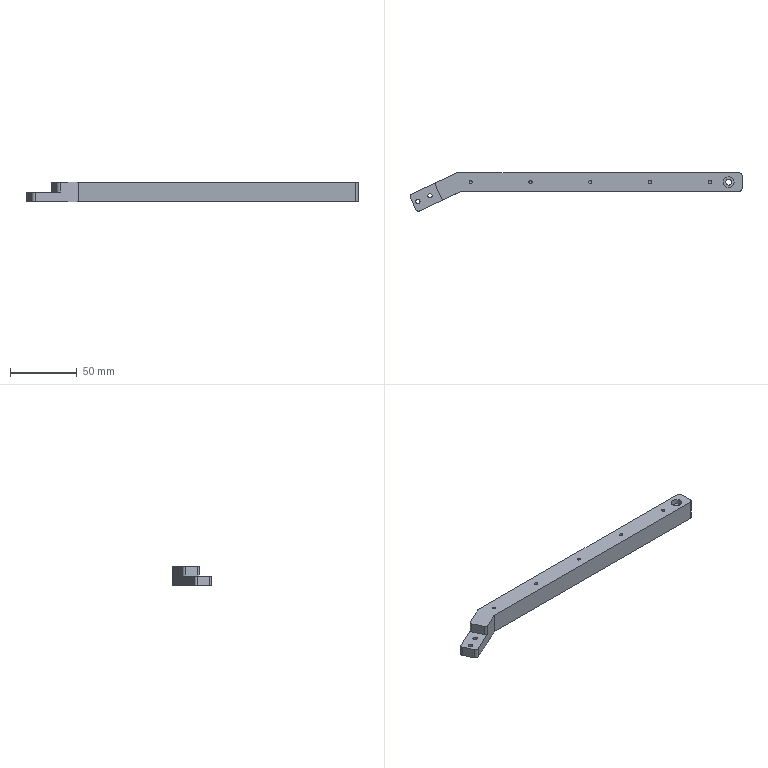Part | NX | 1 solid | 33 faces | box 249.594 x 28.935 x 15 mm | volume 49736 mm3 | cylinder 17 | plane 11 | cone 5 | commonest cylinder face diameters 4 x8 2.459 x5 3.242 x2 4.5 x1 8 x1
STEP:
#1=CARTESIAN_POINT('',(-120.493,-7.091,-15.));
#2=VERTEX_POINT('',#1);
#3=CARTESIAN_POINT('',(-118.872,-7.091,-15.));
#4=DIRECTION('',(0.,0.,1.));
#5=DIRECTION('',(-1.,0.,0.));
#6=AXIS2_PLACEMENT_3D('',#3,#4,#5);
#7=CIRCLE('',#6,1.621);
#8=EDGE_CURVE('',#2,#2,#7,.T.);
#9=ORIENTED_EDGE('',*,*,#8,.F.);
#10=EDGE_LOOP('',(#9));
#11=FACE_BOUND('',#10,.T.);
#12=CARTESIAN_POINT('',(-120.493,-7.091,-7.5));
#13=VERTEX_POINT('',#12);
#14=CARTESIAN_POINT('',(-118.872,-7.091,-7.5));
#15=DIRECTION('',(0.,0.,1.));
#16=DIRECTION('',(-1.,0.,0.));
#17=AXIS2_PLACEMENT_3D('',#14,#15,#16);
#18=CIRCLE('',#17,1.621);
#19=EDGE_CURVE('',#13,#13,#18,.T.);
#20=ORIENTED_EDGE('',*,*,#19,.T.);
#21=EDGE_LOOP('',(#20));
#22=FACE_BOUND('',#21,.T.);
#23=CARTESIAN_POINT('',(-118.872,-7.091,-7.5));
#24=DIRECTION('',(0.,0.,-1.));
#25=DIRECTION('',(0.,-1.,0.));
#26=AXIS2_PLACEMENT_3D('',#23,#24,#25);
#27=CYLINDRICAL_SURFACE('',#26,1.621);
#28=ADVANCED_FACE('',(#11,#22),#27,.F.);
#29=CARTESIAN_POINT('',(117.047,7.468,-15.));
#30=VERTEX_POINT('',#29);
#31=CARTESIAN_POINT('',(114.797,7.468,-15.));
#32=DIRECTION('',(0.,0.,-1.));
#33=DIRECTION('',(1.,0.,0.));
#34=AXIS2_PLACEMENT_3D('',#31,#32,#33);
#35=CIRCLE('',#34,2.25);
#36=EDGE_CURVE('',#30,#30,#35,.T.);
#37=ORIENTED_EDGE('',*,*,#36,.F.);
#38=EDGE_LOOP('',(#37));
#39=FACE_BOUND('',#38,.T.);
#40=CARTESIAN_POINT('',(-108.187,-2.865,-15.));
#41=VERTEX_POINT('',#40);
#42=CARTESIAN_POINT('',(-109.808,-2.865,-15.));
#43=DIRECTION('',(0.,0.,-1.));
#44=DIRECTION('',(1.,0.,0.));
#45=AXIS2_PLACEMENT_3D('',#42,#43,#44);
#46=CIRCLE('',#45,1.621);
#47=EDGE_CURVE('',#41,#41,#46,.T.);
#48=ORIENTED_EDGE('',*,*,#47,.F.);
#49=EDGE_LOOP('',(#48));
#50=FACE_BOUND('',#49,.T.);
#51=ORIENTED_EDGE('',*,*,#8,.T.);
#52=EDGE_LOOP('',(#51));
#53=FACE_BOUND('',#52,.T.);
#54=CARTESIAN_POINT('',(-86.501,0.2802,-15.));
#55=VERTEX_POINT('',#54);
#56=CARTESIAN_POINT('',(-117.726,-14.28,-15.));
#57=VERTEX_POINT('',#56);
#58=CARTESIAN_POINT('',(-102.113,-7.,-15.));
#59=DIRECTION('',(-0.9063,-0.4226,0.));
#60=VECTOR('',#59,1000.);
#61=LINE('',#58,#60);
#62=EDGE_CURVE('',#55,#57,#61,.T.);
#63=ORIENTED_EDGE('',*,*,#62,.T.);
#64=CARTESIAN_POINT('',(-120.384,-13.313,-15.));
#65=VERTEX_POINT('',#64);
#66=CARTESIAN_POINT('',(-118.571,-12.468,-15.));
#67=DIRECTION('',(0.,0.,-1.));
#68=DIRECTION('',(1.,0.,0.));
#69=AXIS2_PLACEMENT_3D('',#66,#67,#68);
#70=CIRCLE('',#69,2.);
#71=EDGE_CURVE('',#57,#65,#70,.T.);
#72=ORIENTED_EDGE('',*,*,#71,.T.);
#73=CARTESIAN_POINT('',(-124.61,-4.25,-15.));
#74=VERTEX_POINT('',#73);
#75=CARTESIAN_POINT('',(-122.497,-8.781,-15.));
#76=DIRECTION('',(0.4226,-0.9063,0.));
#77=VECTOR('',#76,1000.);
#78=LINE('',#75,#77);
#79=EDGE_CURVE('',#74,#65,#78,.T.);
#80=ORIENTED_EDGE('',*,*,#79,.F.);
#81=CARTESIAN_POINT('',(-123.642,-1.592,-15.));
#82=VERTEX_POINT('',#81);
#83=CARTESIAN_POINT('',(-122.797,-3.405,-15.));
#84=DIRECTION('',(0.,0.,-1.));
#85=DIRECTION('',(1.,0.,0.));
#86=AXIS2_PLACEMENT_3D('',#83,#84,#85);
#87=CIRCLE('',#86,2.);
#88=EDGE_CURVE('',#74,#82,#87,.T.);
#89=ORIENTED_EDGE('',*,*,#88,.T.);
#90=CARTESIAN_POINT('',(-89.605,14.28,-15.));
#91=VERTEX_POINT('',#90);
#92=CARTESIAN_POINT('',(-106.624,6.344,-15.));
#93=DIRECTION('',(0.9063,0.4226,0.));
#94=VECTOR('',#93,1000.);
#95=LINE('',#92,#94);
#96=EDGE_CURVE('',#82,#91,#95,.T.);
#97=ORIENTED_EDGE('',*,*,#96,.T.);
#98=CARTESIAN_POINT('',(-88.759,14.468,-15.));
#99=VERTEX_POINT('',#98);
#100=CARTESIAN_POINT('',(-88.759,12.468,-15.));
#101=DIRECTION('',(0.,0.,1.));
#102=DIRECTION('',(-1.,0.,0.));
#103=AXIS2_PLACEMENT_3D('',#100,#101,#102);
#104=CIRCLE('',#103,2.);
#105=EDGE_CURVE('',#99,#91,#104,.T.);
#106=ORIENTED_EDGE('',*,*,#105,.F.);
#107=CARTESIAN_POINT('',(122.797,14.468,-15.));
#108=VERTEX_POINT('',#107);
#109=CARTESIAN_POINT('',(17.019,14.468,-15.));
#110=DIRECTION('',(-1.,0.,0.));
#111=VECTOR('',#110,1000.);
#112=LINE('',#109,#111);
#113=EDGE_CURVE('',#108,#99,#112,.T.);
#114=ORIENTED_EDGE('',*,*,#113,.F.);
#115=CARTESIAN_POINT('',(124.797,12.468,-15.));
#116=VERTEX_POINT('',#115);
#117=CARTESIAN_POINT('',(122.797,12.468,-15.));
#118=DIRECTION('',(0.,0.,1.));
#119=DIRECTION('',(-1.,0.,0.));
#120=AXIS2_PLACEMENT_3D('',#117,#118,#119);
#121=CIRCLE('',#120,2.);
#122=EDGE_CURVE('',#116,#108,#121,.T.);
#123=ORIENTED_EDGE('',*,*,#122,.F.);
#124=CARTESIAN_POINT('',(124.797,2.468,-15.));
#125=VERTEX_POINT('',#124);
#126=CARTESIAN_POINT('',(124.797,7.468,-15.));
#127=DIRECTION('',(0.,1.,0.));
#128=VECTOR('',#127,1000.);
#129=LINE('',#126,#128);
#130=EDGE_CURVE('',#125,#116,#129,.T.);
#131=ORIENTED_EDGE('',*,*,#130,.F.);
#132=CARTESIAN_POINT('',(122.797,0.4676,-15.));
#133=VERTEX_POINT('',#132);
#134=CARTESIAN_POINT('',(122.797,2.468,-15.));
#135=DIRECTION('',(0.,0.,1.));
#136=DIRECTION('',(-1.,0.,0.));
#137=AXIS2_PLACEMENT_3D('',#134,#135,#136);
#138=CIRCLE('',#137,2.);
#139=EDGE_CURVE('',#133,#125,#138,.T.);
#140=ORIENTED_EDGE('',*,*,#139,.F.);
#141=CARTESIAN_POINT('',(-85.656,0.4676,-15.));
#142=VERTEX_POINT('',#141);
#143=CARTESIAN_POINT('',(18.571,0.4676,-15.));
#144=DIRECTION('',(1.,0.,0.));
#145=VECTOR('',#144,1000.);
#146=LINE('',#143,#145);
#147=EDGE_CURVE('',#142,#133,#146,.T.);
#148=ORIENTED_EDGE('',*,*,#147,.F.);
#149=CARTESIAN_POINT('',(-85.656,-1.532,-15.));
#150=DIRECTION('',(0.,0.,-1.));
#151=DIRECTION('',(1.,0.,0.));
#152=AXIS2_PLACEMENT_3D('',#149,#150,#151);
#153=CIRCLE('',#152,2.);
#154=EDGE_CURVE('',#55,#142,#153,.T.);
#155=ORIENTED_EDGE('',*,*,#154,.F.);
#156=EDGE_LOOP('',(#63,#72,#80,#89,#97,#106,#114,#123,#131,#140,#148,#155));
#157=FACE_BOUND('',#156,.T.);
#158=CARTESIAN_POINT('',(-89.203,14.468,-15.));
#159=DIRECTION('',(0.,0.,1.));
#160=DIRECTION('',(0.,-1.,0.));
#161=AXIS2_PLACEMENT_3D('',#158,#159,#160);
#162=PLANE('',#161);
#163=ADVANCED_FACE('',(#39,#50,#53,#157),#162,.F.);
#164=ORIENTED_EDGE('',*,*,#147,.T.);
#165=CARTESIAN_POINT('',(122.797,0.4676,0.));
#166=VERTEX_POINT('',#165);
#167=CARTESIAN_POINT('',(122.797,0.4676,-7.5));
#168=DIRECTION('',(0.,0.,1.));
#169=VECTOR('',#168,1000.);
#170=LINE('',#167,#169);
#171=EDGE_CURVE('',#133,#166,#170,.T.);
#172=ORIENTED_EDGE('',*,*,#171,.T.);
#173=CARTESIAN_POINT('',(-85.656,0.4676,0.));
#174=VERTEX_POINT('',#173);
#175=CARTESIAN_POINT('',(18.571,0.4676,0.));
#176=DIRECTION('',(1.,0.,0.));
#177=VECTOR('',#176,1000.);
#178=LINE('',#175,#177);
#179=EDGE_CURVE('',#174,#166,#178,.T.);
#180=ORIENTED_EDGE('',*,*,#179,.F.);
#181=CARTESIAN_POINT('',(-85.656,0.4676,-7.5));
#182=DIRECTION('',(0.,0.,-1.));
#183=VECTOR('',#182,1000.);
#184=LINE('',#181,#183);
#185=EDGE_CURVE('',#174,#142,#184,.T.);
#186=ORIENTED_EDGE('',*,*,#185,.T.);
#187=EDGE_LOOP('',(#164,#172,#180,#186));
#188=FACE_BOUND('',#187,.T.);
#189=CARTESIAN_POINT('',(-89.203,0.4676,-15.));
#190=DIRECTION('',(0.,-1.,0.));
#191=DIRECTION('',(1.,0.,0.));
#192=AXIS2_PLACEMENT_3D('',#189,#190,#191);
#193=PLANE('',#192);
#194=ADVANCED_FACE('',(#188),#193,.T.);
#195=CARTESIAN_POINT('',(102.027,7.468,0.));
#196=VERTEX_POINT('',#195);
#197=CARTESIAN_POINT('',(100.797,7.468,0.));
#198=DIRECTION('',(0.,0.,-1.));
#199=DIRECTION('',(1.,0.,0.));
#200=AXIS2_PLACEMENT_3D('',#197,#198,#199);
#201=CIRCLE('',#200,1.23);
#202=EDGE_CURVE('',#196,#196,#201,.T.);
#203=ORIENTED_EDGE('',*,*,#202,.T.);
#204=EDGE_LOOP('',(#203));
#205=FACE_BOUND('',#204,.T.);
#206=CARTESIAN_POINT('',(57.027,7.468,0.));
#207=VERTEX_POINT('',#206);
#208=CARTESIAN_POINT('',(55.797,7.468,0.));
#209=DIRECTION('',(0.,0.,-1.));
#210=DIRECTION('',(1.,0.,0.));
#211=AXIS2_PLACEMENT_3D('',#208,#209,#210);
#212=CIRCLE('',#211,1.23);
#213=EDGE_CURVE('',#207,#207,#212,.T.);
#214=ORIENTED_EDGE('',*,*,#213,.T.);
#215=EDGE_LOOP('',(#214));
#216=FACE_BOUND('',#215,.T.);
#217=CARTESIAN_POINT('',(12.027,7.468,0.));
#218=VERTEX_POINT('',#217);
#219=CARTESIAN_POINT('',(10.797,7.468,0.));
#220=DIRECTION('',(0.,0.,-1.));
#221=DIRECTION('',(1.,0.,0.));
#222=AXIS2_PLACEMENT_3D('',#219,#220,#221);
#223=CIRCLE('',#222,1.23);
#224=EDGE_CURVE('',#218,#218,#223,.T.);
#225=ORIENTED_EDGE('',*,*,#224,.T.);
#226=EDGE_LOOP('',(#225));
#227=FACE_BOUND('',#226,.T.);
#228=CARTESIAN_POINT('',(-32.973,7.468,0.));
#229=VERTEX_POINT('',#228);
#230=CARTESIAN_POINT('',(-34.203,7.468,0.));
#231=DIRECTION('',(0.,0.,-1.));
#232=DIRECTION('',(1.,0.,0.));
#233=AXIS2_PLACEMENT_3D('',#230,#231,#232);
#234=CIRCLE('',#233,1.23);
#235=EDGE_CURVE('',#229,#229,#234,.T.);
#236=ORIENTED_EDGE('',*,*,#235,.T.);
#237=EDGE_LOOP('',(#236));
#238=FACE_BOUND('',#237,.T.);
#239=CARTESIAN_POINT('',(118.797,7.468,0.));
#240=VERTEX_POINT('',#239);
#241=CARTESIAN_POINT('',(114.797,7.468,0.));
#242=DIRECTION('',(0.,0.,-1.));
#243=DIRECTION('',(1.,0.,0.));
#244=AXIS2_PLACEMENT_3D('',#241,#242,#243);
#245=CIRCLE('',#244,4.);
#246=EDGE_CURVE('',#240,#240,#245,.T.);
#247=ORIENTED_EDGE('',*,*,#246,.T.);
#248=EDGE_LOOP('',(#247));
#249=FACE_BOUND('',#248,.T.);
#250=CARTESIAN_POINT('',(-77.973,7.468,0.));
#251=VERTEX_POINT('',#250);
#252=CARTESIAN_POINT('',(-79.203,7.468,0.));
#253=DIRECTION('',(0.,0.,-1.));
#254=DIRECTION('',(1.,0.,0.));
#255=AXIS2_PLACEMENT_3D('',#252,#253,#254);
#256=CIRCLE('',#255,1.23);
#257=EDGE_CURVE('',#251,#251,#256,.T.);
#258=ORIENTED_EDGE('',*,*,#257,.T.);
#259=EDGE_LOOP('',(#258));
#260=FACE_BOUND('',#259,.T.);
#261=CARTESIAN_POINT('',(-86.501,0.2802,0.));
#262=VERTEX_POINT('',#261);
#263=CARTESIAN_POINT('',(-85.656,-1.532,0.));
#264=DIRECTION('',(0.,0.,-1.));
#265=DIRECTION('',(1.,0.,0.));
#266=AXIS2_PLACEMENT_3D('',#263,#264,#265);
#267=CIRCLE('',#266,2.);
#268=EDGE_CURVE('',#262,#174,#267,.T.);
#269=ORIENTED_EDGE('',*,*,#268,.T.);
#270=ORIENTED_EDGE('',*,*,#179,.T.);
#271=CARTESIAN_POINT('',(124.797,2.468,0.));
#272=VERTEX_POINT('',#271);
#273=CARTESIAN_POINT('',(122.797,2.468,0.));
#274=DIRECTION('',(0.,0.,1.));
#275=DIRECTION('',(-1.,0.,0.));
#276=AXIS2_PLACEMENT_3D('',#273,#274,#275);
#277=CIRCLE('',#276,2.);
#278=EDGE_CURVE('',#166,#272,#277,.T.);
#279=ORIENTED_EDGE('',*,*,#278,.T.);
#280=CARTESIAN_POINT('',(124.797,12.468,0.));
#281=VERTEX_POINT('',#280);
#282=CARTESIAN_POINT('',(124.797,7.468,0.));
#283=DIRECTION('',(0.,1.,0.));
#284=VECTOR('',#283,1000.);
#285=LINE('',#282,#284);
#286=EDGE_CURVE('',#272,#281,#285,.T.);
#287=ORIENTED_EDGE('',*,*,#286,.T.);
#288=CARTESIAN_POINT('',(122.797,14.468,0.));
#289=VERTEX_POINT('',#288);
#290=CARTESIAN_POINT('',(122.797,12.468,0.));
#291=DIRECTION('',(0.,0.,1.));
#292=DIRECTION('',(-1.,0.,0.));
#293=AXIS2_PLACEMENT_3D('',#290,#291,#292);
#294=CIRCLE('',#293,2.);
#295=EDGE_CURVE('',#281,#289,#294,.T.);
#296=ORIENTED_EDGE('',*,*,#295,.T.);
#297=CARTESIAN_POINT('',(-88.759,14.468,0.));
#298=VERTEX_POINT('',#297);
#299=CARTESIAN_POINT('',(17.019,14.468,0.));
#300=DIRECTION('',(-1.,0.,0.));
#301=VECTOR('',#300,1000.);
#302=LINE('',#299,#301);
#303=EDGE_CURVE('',#289,#298,#302,.T.);
#304=ORIENTED_EDGE('',*,*,#303,.T.);
#305=CARTESIAN_POINT('',(-89.605,14.28,0.));
#306=VERTEX_POINT('',#305);
#307=CARTESIAN_POINT('',(-88.759,12.468,0.));
#308=DIRECTION('',(0.,0.,1.));
#309=DIRECTION('',(-1.,0.,0.));
#310=AXIS2_PLACEMENT_3D('',#307,#308,#309);
#311=CIRCLE('',#310,2.);
#312=EDGE_CURVE('',#298,#306,#311,.T.);
#313=ORIENTED_EDGE('',*,*,#312,.T.);
#314=CARTESIAN_POINT('',(-104.61,7.283,0.));
#315=VERTEX_POINT('',#314);
#316=CARTESIAN_POINT('',(-97.107,10.782,0.));
#317=DIRECTION('',(0.9063,0.4226,0.));
#318=VECTOR('',#317,1000.);
#319=LINE('',#316,#318);
#320=EDGE_CURVE('',#315,#306,#319,.T.);
#321=ORIENTED_EDGE('',*,*,#320,.F.);
#322=CARTESIAN_POINT('',(-105.577,4.625,0.));
#323=VERTEX_POINT('',#322);
#324=CARTESIAN_POINT('',(-103.765,5.47,0.));
#325=DIRECTION('',(0.,0.,-1.));
#326=DIRECTION('',(1.,0.,0.));
#327=AXIS2_PLACEMENT_3D('',#324,#325,#326);
#328=CIRCLE('',#327,2.);
#329=EDGE_CURVE('',#323,#315,#328,.T.);
#330=ORIENTED_EDGE('',*,*,#329,.F.);
#331=CARTESIAN_POINT('',(-101.351,-4.438,0.));
#332=VERTEX_POINT('',#331);
#333=CARTESIAN_POINT('',(-103.464,0.09369,0.));
#334=DIRECTION('',(0.4226,-0.9063,0.));
#335=VECTOR('',#334,1000.);
#336=LINE('',#333,#335);
#337=EDGE_CURVE('',#323,#332,#336,.T.);
#338=ORIENTED_EDGE('',*,*,#337,.T.);
#339=CARTESIAN_POINT('',(-98.693,-5.405,0.));
#340=VERTEX_POINT('',#339);
#341=CARTESIAN_POINT('',(-99.539,-3.593,0.));
#342=DIRECTION('',(0.,0.,-1.));
#343=DIRECTION('',(1.,0.,0.));
#344=AXIS2_PLACEMENT_3D('',#341,#342,#343);
#345=CIRCLE('',#344,2.);
#346=EDGE_CURVE('',#340,#332,#345,.T.);
#347=ORIENTED_EDGE('',*,*,#346,.F.);
#348=CARTESIAN_POINT('',(-92.597,-2.563,0.));
#349=DIRECTION('',(-0.9063,-0.4226,0.));
#350=VECTOR('',#349,1000.);
#351=LINE('',#348,#350);
#352=EDGE_CURVE('',#262,#340,#351,.T.);
#353=ORIENTED_EDGE('',*,*,#352,.F.);
#354=EDGE_LOOP('',(#269,#270,#279,#287,#296,#304,#313,#321,#330,#338,#347,#353));
#355=FACE_BOUND('',#354,.T.);
#356=CARTESIAN_POINT('',(-89.203,14.468,0.));
#357=DIRECTION('',(0.,0.,1.));
#358=DIRECTION('',(0.,-1.,0.));
#359=AXIS2_PLACEMENT_3D('',#356,#357,#358);
#360=PLANE('',#359);
#361=ADVANCED_FACE('',(#205,#216,#227,#238,#249,#260,#355),#360,.T.);
#362=ORIENTED_EDGE('',*,*,#278,.F.);
#363=ORIENTED_EDGE('',*,*,#171,.F.);
#364=ORIENTED_EDGE('',*,*,#139,.T.);
#365=CARTESIAN_POINT('',(124.797,2.468,-7.5));
#366=DIRECTION('',(0.,0.,1.));
#367=VECTOR('',#366,1000.);
#368=LINE('',#365,#367);
#369=EDGE_CURVE('',#125,#272,#368,.T.);
#370=ORIENTED_EDGE('',*,*,#369,.T.);
#371=EDGE_LOOP('',(#362,#363,#364,#370));
#372=FACE_BOUND('',#371,.T.);
#373=CARTESIAN_POINT('',(122.797,2.468,-7.5));
#374=DIRECTION('',(0.,0.,1.));
#375=DIRECTION('',(0.,-1.,0.));
#376=AXIS2_PLACEMENT_3D('',#373,#374,#375);
#377=CYLINDRICAL_SURFACE('',#376,2.);
#378=ADVANCED_FACE('',(#372),#377,.T.);
#379=ORIENTED_EDGE('',*,*,#130,.T.);
#380=CARTESIAN_POINT('',(124.797,12.468,-7.5));
#381=DIRECTION('',(0.,0.,1.));
#382=VECTOR('',#381,1000.);
#383=LINE('',#380,#382);
#384=EDGE_CURVE('',#116,#281,#383,.T.);
#385=ORIENTED_EDGE('',*,*,#384,.T.);
#386=ORIENTED_EDGE('',*,*,#286,.F.);
#387=ORIENTED_EDGE('',*,*,#369,.F.);
#388=EDGE_LOOP('',(#379,#385,#386,#387));
#389=FACE_BOUND('',#388,.T.);
#390=CARTESIAN_POINT('',(124.797,0.4676,-15.));
#391=DIRECTION('',(1.,0.,0.));
#392=DIRECTION('',(0.,1.,0.));
#393=AXIS2_PLACEMENT_3D('',#390,#391,#392);
#394=PLANE('',#393);
#395=ADVANCED_FACE('',(#389),#394,.T.);
#396=CARTESIAN_POINT('',(117.047,7.468,-4.));
#397=VERTEX_POINT('',#396);
#398=CARTESIAN_POINT('',(114.797,7.468,-4.));
#399=DIRECTION('',(0.,0.,-1.));
#400=DIRECTION('',(1.,0.,0.));
#401=AXIS2_PLACEMENT_3D('',#398,#399,#400);
#402=CIRCLE('',#401,2.25);
#403=EDGE_CURVE('',#397,#397,#402,.T.);
#404=ORIENTED_EDGE('',*,*,#403,.T.);
#405=EDGE_LOOP('',(#404));
#406=FACE_BOUND('',#405,.T.);
#407=CARTESIAN_POINT('',(118.797,7.468,-4.));
#408=VERTEX_POINT('',#407);
#409=CARTESIAN_POINT('',(114.797,7.468,-4.));
#410=DIRECTION('',(0.,0.,-1.));
#411=DIRECTION('',(1.,0.,0.));
#412=AXIS2_PLACEMENT_3D('',#409,#410,#411);
#413=CIRCLE('',#412,4.);
#414=EDGE_CURVE('',#408,#408,#413,.T.);
#415=ORIENTED_EDGE('',*,*,#414,.F.);
#416=EDGE_LOOP('',(#415));
#417=FACE_BOUND('',#416,.T.);
#418=CARTESIAN_POINT('',(114.797,5.218,-4.));
#419=DIRECTION('',(0.,0.,-1.));
#420=DIRECTION('',(0.,-1.,0.));
#421=AXIS2_PLACEMENT_3D('',#418,#419,#420);
#422=PLANE('',#421);
#423=ADVANCED_FACE('',(#406,#417),#422,.F.);
#424=CARTESIAN_POINT('',(-80.432,7.468,-8.));
#425=VERTEX_POINT('',#424);
#426=CARTESIAN_POINT('',(-79.203,7.468,-8.));
#427=DIRECTION('',(0.,0.,1.));
#428=DIRECTION('',(-1.,0.,0.));
#429=AXIS2_PLACEMENT_3D('',#426,#427,#428);
#430=CIRCLE('',#429,1.23);
#431=EDGE_CURVE('',#425,#425,#430,.T.);
#432=ORIENTED_EDGE('',*,*,#431,.F.);
#433=EDGE_LOOP('',(#432));
#434=FACE_BOUND('',#433,.T.);
#435=ORIENTED_EDGE('',*,*,#257,.F.);
#436=EDGE_LOOP('',(#435));
#437=FACE_BOUND('',#436,.T.);
#438=CARTESIAN_POINT('',(-79.203,7.468,0.));
#439=DIRECTION('',(0.,0.,-1.));
#440=DIRECTION('',(0.,-1.,0.));
#441=AXIS2_PLACEMENT_3D('',#438,#439,#440);
#442=CYLINDRICAL_SURFACE('',#441,1.23);
#443=ADVANCED_FACE('',(#434,#437),#442,.F.);
#444=ORIENTED_EDGE('',*,*,#414,.T.);
#445=EDGE_LOOP('',(#444));
#446=FACE_BOUND('',#445,.T.);
#447=ORIENTED_EDGE('',*,*,#246,.F.);
#448=EDGE_LOOP('',(#447));
#449=FACE_BOUND('',#448,.T.);
#450=CARTESIAN_POINT('',(114.797,7.468,0.));
#451=DIRECTION('',(0.,0.,-1.));
#452=DIRECTION('',(0.,-1.,0.));
#453=AXIS2_PLACEMENT_3D('',#450,#451,#452);
#454=CYLINDRICAL_SURFACE('',#453,4.);
#455=ADVANCED_FACE('',(#446,#449),#454,.F.);
#456=CARTESIAN_POINT('',(-35.432,7.468,-8.));
#457=VERTEX_POINT('',#456);
#458=CARTESIAN_POINT('',(-34.203,7.468,-8.));
#459=DIRECTION('',(0.,0.,1.));
#460=DIRECTION('',(-1.,0.,0.));
#461=AXIS2_PLACEMENT_3D('',#458,#459,#460);
#462=CIRCLE('',#461,1.23);
#463=EDGE_CURVE('',#457,#457,#462,.T.);
#464=ORIENTED_EDGE('',*,*,#463,.F.);
#465=EDGE_LOOP('',(#464));
#466=FACE_BOUND('',#465,.T.);
#467=ORIENTED_EDGE('',*,*,#235,.F.);
#468=EDGE_LOOP('',(#467));
#469=FACE_BOUND('',#468,.T.);
#470=CARTESIAN_POINT('',(-34.203,7.468,0.));
#471=DIRECTION('',(0.,0.,-1.));
#472=DIRECTION('',(0.,-1.,0.));
#473=AXIS2_PLACEMENT_3D('',#470,#471,#472);
#474=CYLINDRICAL_SURFACE('',#473,1.23);
#475=ADVANCED_FACE('',(#466,#469),#474,.F.);
#476=CARTESIAN_POINT('',(9.568,7.468,-8.));
#477=VERTEX_POINT('',#476);
#478=CARTESIAN_POINT('',(10.797,7.468,-8.));
#479=DIRECTION('',(0.,0.,1.));
#480=DIRECTION('',(-1.,0.,0.));
#481=AXIS2_PLACEMENT_3D('',#478,#479,#480);
#482=CIRCLE('',#481,1.23);
#483=EDGE_CURVE('',#477,#477,#482,.T.);
#484=ORIENTED_EDGE('',*,*,#483,.F.);
#485=EDGE_LOOP('',(#484));
#486=FACE_BOUND('',#485,.T.);
#487=ORIENTED_EDGE('',*,*,#224,.F.);
#488=EDGE_LOOP('',(#487));
#489=FACE_BOUND('',#488,.T.);
#490=CARTESIAN_POINT('',(10.797,7.468,0.));
#491=DIRECTION('',(0.,0.,-1.));
#492=DIRECTION('',(0.,-1.,0.));
#493=AXIS2_PLACEMENT_3D('',#490,#491,#492);
#494=CYLINDRICAL_SURFACE('',#493,1.23);
#495=ADVANCED_FACE('',(#486,#489),#494,.F.);
#496=CARTESIAN_POINT('',(54.568,7.468,-8.));
#497=VERTEX_POINT('',#496);
#498=CARTESIAN_POINT('',(55.797,7.468,-8.));
#499=DIRECTION('',(0.,0.,1.));
#500=DIRECTION('',(-1.,0.,0.));
#501=AXIS2_PLACEMENT_3D('',#498,#499,#500);
#502=CIRCLE('',#501,1.23);
#503=EDGE_CURVE('',#497,#497,#502,.T.);
#504=ORIENTED_EDGE('',*,*,#503,.F.);
#505=EDGE_LOOP('',(#504));
#506=FACE_BOUND('',#505,.T.);
#507=ORIENTED_EDGE('',*,*,#213,.F.);
#508=EDGE_LOOP('',(#507));
#509=FACE_BOUND('',#508,.T.);
#510=CARTESIAN_POINT('',(55.797,7.468,0.));
#511=DIRECTION('',(0.,0.,-1.));
#512=DIRECTION('',(0.,-1.,0.));
#513=AXIS2_PLACEMENT_3D('',#510,#511,#512);
#514=CYLINDRICAL_SURFACE('',#513,1.23);
#515=ADVANCED_FACE('',(#506,#509),#514,.F.);
#516=CARTESIAN_POINT('',(99.568,7.468,-8.));
#517=VERTEX_POINT('',#516);
#518=CARTESIAN_POINT('',(100.797,7.468,-8.));
#519=DIRECTION('',(0.,0.,1.));
#520=DIRECTION('',(-1.,0.,0.));
#521=AXIS2_PLACEMENT_3D('',#518,#519,#520);
#522=CIRCLE('',#521,1.23);
#523=EDGE_CURVE('',#517,#517,#522,.T.);
#524=ORIENTED_EDGE('',*,*,#523,.F.);
#525=EDGE_LOOP('',(#524));
#526=FACE_BOUND('',#525,.T.);
#527=ORIENTED_EDGE('',*,*,#202,.F.);
#528=EDGE_LOOP('',(#527));
#529=FACE_BOUND('',#528,.T.);
#530=CARTESIAN_POINT('',(100.797,7.468,0.));
#531=DIRECTION('',(0.,0.,-1.));
#532=DIRECTION('',(0.,-1.,0.));
#533=AXIS2_PLACEMENT_3D('',#530,#531,#532);
#534=CYLINDRICAL_SURFACE('',#533,1.23);
#535=ADVANCED_FACE('',(#526,#529),#534,.F.);
#536=ORIENTED_EDGE('',*,*,#523,.T.);
#537=EDGE_LOOP('',(#536));
#538=FACE_BOUND('',#537,.T.);
#539=CARTESIAN_POINT('',(100.797,7.468,-8.71));
#540=VERTEX_POINT('',#539);
#541=VERTEX_LOOP('',#540);
#542=FACE_BOUND('',#541,.T.);
#543=CARTESIAN_POINT('',(100.797,7.468,-8.71));
#544=DIRECTION('',(0.,0.,1.));
#545=DIRECTION('',(0.,-1.,0.));
#546=AXIS2_PLACEMENT_3D('',#543,#544,#545);
#547=CONICAL_SURFACE('',#546,0.,1.047);
#548=ADVANCED_FACE('',(#538,#542),#547,.F.);
#549=ORIENTED_EDGE('',*,*,#503,.T.);
#550=EDGE_LOOP('',(#549));
#551=FACE_BOUND('',#550,.T.);
#552=CARTESIAN_POINT('',(55.797,7.468,-8.71));
#553=VERTEX_POINT('',#552);
#554=VERTEX_LOOP('',#553);
#555=FACE_BOUND('',#554,.T.);
#556=CARTESIAN_POINT('',(55.797,7.468,-8.71));
#557=DIRECTION('',(0.,0.,1.));
#558=DIRECTION('',(0.,-1.,0.));
#559=AXIS2_PLACEMENT_3D('',#556,#557,#558);
#560=CONICAL_SURFACE('',#559,0.,1.047);
#561=ADVANCED_FACE('',(#551,#555),#560,.F.);
#562=ORIENTED_EDGE('',*,*,#483,.T.);
#563=EDGE_LOOP('',(#562));
#564=FACE_BOUND('',#563,.T.);
#565=CARTESIAN_POINT('',(10.797,7.468,-8.71));
#566=VERTEX_POINT('',#565);
#567=VERTEX_LOOP('',#566);
#568=FACE_BOUND('',#567,.T.);
#569=CARTESIAN_POINT('',(10.797,7.468,-8.71));
#570=DIRECTION('',(0.,0.,1.));
#571=DIRECTION('',(0.,-1.,0.));
#572=AXIS2_PLACEMENT_3D('',#569,#570,#571);
#573=CONICAL_SURFACE('',#572,0.,1.047);
#574=ADVANCED_FACE('',(#564,#568),#573,.F.);
#575=ORIENTED_EDGE('',*,*,#463,.T.);
#576=EDGE_LOOP('',(#575));
#577=FACE_BOUND('',#576,.T.);
#578=CARTESIAN_POINT('',(-34.203,7.468,-8.71));
#579=VERTEX_POINT('',#578);
#580=VERTEX_LOOP('',#579);
#581=FACE_BOUND('',#580,.T.);
#582=CARTESIAN_POINT('',(-34.203,7.468,-8.71));
#583=DIRECTION('',(0.,0.,1.));
#584=DIRECTION('',(0.,-1.,0.));
#585=AXIS2_PLACEMENT_3D('',#582,#583,#584);
#586=CONICAL_SURFACE('',#585,0.,1.047);
#587=ADVANCED_FACE('',(#577,#581),#586,.F.);
#588=ORIENTED_EDGE('',*,*,#431,.T.);
#589=EDGE_LOOP('',(#588));
#590=FACE_BOUND('',#589,.T.);
#591=CARTESIAN_POINT('',(-79.203,7.468,-8.71));
#592=VERTEX_POINT('',#591);
#593=VERTEX_LOOP('',#592);
#594=FACE_BOUND('',#593,.T.);
#595=CARTESIAN_POINT('',(-79.203,7.468,-8.71));
#596=DIRECTION('',(0.,0.,1.));
#597=DIRECTION('',(0.,-1.,0.));
#598=AXIS2_PLACEMENT_3D('',#595,#596,#597);
#599=CONICAL_SURFACE('',#598,0.,1.047);
#600=ADVANCED_FACE('',(#590,#594),#599,.F.);
#601=ORIENTED_EDGE('',*,*,#36,.T.);
#602=EDGE_LOOP('',(#601));
#603=FACE_BOUND('',#602,.T.);
#604=ORIENTED_EDGE('',*,*,#403,.F.);
#605=EDGE_LOOP('',(#604));
#606=FACE_BOUND('',#605,.T.);
#607=CARTESIAN_POINT('',(114.797,7.468,0.));
#608=DIRECTION('',(0.,0.,-1.));
#609=DIRECTION('',(0.,-1.,0.));
#610=AXIS2_PLACEMENT_3D('',#607,#608,#609);
#611=CYLINDRICAL_SURFACE('',#610,2.25);
#612=ADVANCED_FACE('',(#603,#606),#611,.F.);
#613=ORIENTED_EDGE('',*,*,#295,.F.);
#614=ORIENTED_EDGE('',*,*,#384,.F.);
#615=ORIENTED_EDGE('',*,*,#122,.T.);
#616=CARTESIAN_POINT('',(122.797,14.468,-7.5));
#617=DIRECTION('',(0.,0.,1.));
#618=VECTOR('',#617,1000.);
#619=LINE('',#616,#618);
#620=EDGE_CURVE('',#108,#289,#619,.T.);
#621=ORIENTED_EDGE('',*,*,#620,.T.);
#622=EDGE_LOOP('',(#613,#614,#615,#621));
#623=FACE_BOUND('',#622,.T.);
#624=CARTESIAN_POINT('',(122.797,12.468,-7.5));
#625=DIRECTION('',(0.,0.,1.));
#626=DIRECTION('',(1.,0.,0.));
#627=AXIS2_PLACEMENT_3D('',#624,#625,#626);
#628=CYLINDRICAL_SURFACE('',#627,2.);
#629=ADVANCED_FACE('',(#623),#628,.T.);
#630=ORIENTED_EDGE('',*,*,#303,.F.);
#631=ORIENTED_EDGE('',*,*,#620,.F.);
#632=ORIENTED_EDGE('',*,*,#113,.T.);
#633=CARTESIAN_POINT('',(-88.759,14.468,-7.5));
#634=DIRECTION('',(0.,0.,1.));
#635=VECTOR('',#634,1000.);
#636=LINE('',#633,#635);
#637=EDGE_CURVE('',#99,#298,#636,.T.);
#638=ORIENTED_EDGE('',*,*,#637,.T.);
#639=EDGE_LOOP('',(#630,#631,#632,#638));
#640=FACE_BOUND('',#639,.T.);
#641=CARTESIAN_POINT('',(124.797,14.468,-15.));
#642=DIRECTION('',(0.,1.,0.));
#643=DIRECTION('',(-1.,0.,0.));
#644=AXIS2_PLACEMENT_3D('',#641,#642,#643);
#645=PLANE('',#644);
#646=ADVANCED_FACE('',(#640),#645,.T.);
#647=ORIENTED_EDGE('',*,*,#105,.T.);
#648=CARTESIAN_POINT('',(-89.605,14.28,-7.5));
#649=DIRECTION('',(0.,0.,1.));
#650=VECTOR('',#649,1000.);
#651=LINE('',#648,#650);
#652=EDGE_CURVE('',#91,#306,#651,.T.);
#653=ORIENTED_EDGE('',*,*,#652,.T.);
#654=ORIENTED_EDGE('',*,*,#312,.F.);
#655=ORIENTED_EDGE('',*,*,#637,.F.);
#656=EDGE_LOOP('',(#647,#653,#654,#655));
#657=FACE_BOUND('',#656,.T.);
#658=CARTESIAN_POINT('',(-88.759,12.468,-7.5));
#659=DIRECTION('',(0.,0.,1.));
#660=DIRECTION('',(0.,1.,0.));
#661=AXIS2_PLACEMENT_3D('',#658,#659,#660);
#662=CYLINDRICAL_SURFACE('',#661,2.);
#663=ADVANCED_FACE('',(#657),#662,.T.);
#664=ORIENTED_EDGE('',*,*,#96,.F.);
#665=CARTESIAN_POINT('',(-123.642,-1.592,-7.5));
#666=VERTEX_POINT('',#665);
#667=CARTESIAN_POINT('',(-123.642,-1.592,-7.5));
#668=DIRECTION('',(0.,0.,-1.));
#669=VECTOR('',#668,1000.);
#670=LINE('',#667,#669);
#671=EDGE_CURVE('',#666,#82,#670,.T.);
#672=ORIENTED_EDGE('',*,*,#671,.F.);
#673=CARTESIAN_POINT('',(-104.61,7.283,-7.5));
#674=VERTEX_POINT('',#673);
#675=CARTESIAN_POINT('',(-114.126,2.846,-7.5));
#676=DIRECTION('',(0.9063,0.4226,0.));
#677=VECTOR('',#676,1000.);
#678=LINE('',#675,#677);
#679=EDGE_CURVE('',#666,#674,#678,.T.);
#680=ORIENTED_EDGE('',*,*,#679,.T.);
#681=CARTESIAN_POINT('',(-104.61,7.283,-7.5));
#682=DIRECTION('',(0.,0.,-1.));
#683=VECTOR('',#682,1000.);
#684=LINE('',#681,#683);
#685=EDGE_CURVE('',#315,#674,#684,.T.);
#686=ORIENTED_EDGE('',*,*,#685,.F.);
#687=ORIENTED_EDGE('',*,*,#320,.T.);
#688=ORIENTED_EDGE('',*,*,#652,.F.);
#689=EDGE_LOOP('',(#664,#672,#680,#686,#687,#688));
#690=FACE_BOUND('',#689,.T.);
#691=CARTESIAN_POINT('',(-125.455,-2.437,0.));
#692=DIRECTION('',(-0.4226,0.9063,0.));
#693=DIRECTION('',(0.9063,0.4226,0.));
#694=AXIS2_PLACEMENT_3D('',#691,#692,#693);
#695=PLANE('',#694);
#696=ADVANCED_FACE('',(#690),#695,.T.);
#697=CARTESIAN_POINT('',(-105.577,4.625,-7.5));
#698=VERTEX_POINT('',#697);
#699=CARTESIAN_POINT('',(-103.765,5.47,-7.5));
#700=DIRECTION('',(0.,0.,1.));
#701=DIRECTION('',(-1.,0.,0.));
#702=AXIS2_PLACEMENT_3D('',#699,#700,#701);
#703=CIRCLE('',#702,2.);
#704=EDGE_CURVE('',#674,#698,#703,.T.);
#705=ORIENTED_EDGE('',*,*,#704,.T.);
#706=CARTESIAN_POINT('',(-105.577,4.625,-3.75));
#707=DIRECTION('',(0.,0.,-1.));
#708=VECTOR('',#707,1000.);
#709=LINE('',#706,#708);
#710=EDGE_CURVE('',#323,#698,#709,.T.);
#711=ORIENTED_EDGE('',*,*,#710,.F.);
#712=ORIENTED_EDGE('',*,*,#329,.T.);
#713=ORIENTED_EDGE('',*,*,#685,.T.);
#714=EDGE_LOOP('',(#705,#711,#712,#713));
#715=FACE_BOUND('',#714,.T.);
#716=CARTESIAN_POINT('',(-103.765,5.47,-7.5));
#717=DIRECTION('',(0.,0.,-1.));
#718=DIRECTION('',(-0.9063,-0.4226,0.));
#719=AXIS2_PLACEMENT_3D('',#716,#717,#718);
#720=CYLINDRICAL_SURFACE('',#719,2.);
#721=ADVANCED_FACE('',(#715),#720,.T.);
#722=CARTESIAN_POINT('',(-101.351,-4.438,-7.5));
#723=VERTEX_POINT('',#722);
#724=CARTESIAN_POINT('',(-101.351,-4.438,-7.5));
#725=DIRECTION('',(0.,0.,-1.));
#726=VECTOR('',#725,1000.);
#727=LINE('',#724,#726);
#728=EDGE_CURVE('',#332,#723,#727,.T.);
#729=ORIENTED_EDGE('',*,*,#728,.F.);
#730=ORIENTED_EDGE('',*,*,#337,.F.);
#731=ORIENTED_EDGE('',*,*,#710,.T.);
#732=CARTESIAN_POINT('',(-103.464,0.09369,-7.5));
#733=DIRECTION('',(0.4226,-0.9063,0.));
#734=VECTOR('',#733,1000.);
#735=LINE('',#732,#734);
#736=EDGE_CURVE('',#698,#723,#735,.T.);
#737=ORIENTED_EDGE('',*,*,#736,.T.);
#738=EDGE_LOOP('',(#729,#730,#731,#737));
#739=FACE_BOUND('',#738,.T.);
#740=CARTESIAN_POINT('',(-106.423,6.438,0.));
#741=DIRECTION('',(0.9063,0.4226,0.));
#742=DIRECTION('',(0.4226,-0.9063,0.));
#743=AXIS2_PLACEMENT_3D('',#740,#741,#742);
#744=PLANE('',#743);
#745=ADVANCED_FACE('',(#739),#744,.F.);
#746=CARTESIAN_POINT('',(-86.501,0.2802,-7.5));
#747=DIRECTION('',(0.,0.,-1.));
#748=VECTOR('',#747,1000.);
#749=LINE('',#746,#748);
#750=EDGE_CURVE('',#262,#55,#749,.T.);
#751=ORIENTED_EDGE('',*,*,#750,.T.);
#752=ORIENTED_EDGE('',*,*,#154,.T.);
#753=ORIENTED_EDGE('',*,*,#185,.F.);
#754=ORIENTED_EDGE('',*,*,#268,.F.);
#755=EDGE_LOOP('',(#751,#752,#753,#754));
#756=FACE_BOUND('',#755,.T.);
#757=CARTESIAN_POINT('',(-85.656,-1.532,-7.5));
#758=DIRECTION('',(0.,0.,-1.));
#759=DIRECTION('',(-0.4226,0.9063,0.));
#760=AXIS2_PLACEMENT_3D('',#757,#758,#759);
#761=CYLINDRICAL_SURFACE('',#760,2.);
#762=ADVANCED_FACE('',(#756),#761,.F.);
#763=CARTESIAN_POINT('',(-98.693,-5.405,-7.5));
#764=VERTEX_POINT('',#763);
#765=CARTESIAN_POINT('',(-99.539,-3.593,-7.5));
#766=DIRECTION('',(0.,0.,1.));
#767=DIRECTION('',(-1.,0.,0.));
#768=AXIS2_PLACEMENT_3D('',#765,#766,#767);
#769=CIRCLE('',#768,2.);
#770=EDGE_CURVE('',#723,#764,#769,.T.);
#771=ORIENTED_EDGE('',*,*,#770,.T.);
#772=CARTESIAN_POINT('',(-98.693,-5.405,-3.75));
#773=DIRECTION('',(0.,0.,-1.));
#774=VECTOR('',#773,1000.);
#775=LINE('',#772,#774);
#776=EDGE_CURVE('',#340,#764,#775,.T.);
#777=ORIENTED_EDGE('',*,*,#776,.F.);
#778=ORIENTED_EDGE('',*,*,#346,.T.);
#779=ORIENTED_EDGE('',*,*,#728,.T.);
#780=EDGE_LOOP('',(#771,#777,#778,#779));
#781=FACE_BOUND('',#780,.T.);
#782=CARTESIAN_POINT('',(-99.539,-3.593,-7.5));
#783=DIRECTION('',(0.,0.,-1.));
#784=DIRECTION('',(0.4226,-0.9063,0.));
#785=AXIS2_PLACEMENT_3D('',#782,#783,#784);
#786=CYLINDRICAL_SURFACE('',#785,2.);
#787=ADVANCED_FACE('',(#781),#786,.T.);
#788=ORIENTED_EDGE('',*,*,#352,.T.);
#789=ORIENTED_EDGE('',*,*,#776,.T.);
#790=CARTESIAN_POINT('',(-117.726,-14.28,-7.5));
#791=VERTEX_POINT('',#790);
#792=CARTESIAN_POINT('',(-108.21,-9.843,-7.5));
#793=DIRECTION('',(-0.9063,-0.4226,0.));
#794=VECTOR('',#793,1000.);
#795=LINE('',#792,#794);
#796=EDGE_CURVE('',#764,#791,#795,.T.);
#797=ORIENTED_EDGE('',*,*,#796,.T.);
#798=CARTESIAN_POINT('',(-117.726,-14.28,-7.5));
#799=DIRECTION('',(0.,0.,-1.));
#800=VECTOR('',#799,1000.);
#801=LINE('',#798,#800);
#802=EDGE_CURVE('',#791,#57,#801,.T.);
#803=ORIENTED_EDGE('',*,*,#802,.T.);
#804=ORIENTED_EDGE('',*,*,#62,.F.);
#805=ORIENTED_EDGE('',*,*,#750,.F.);
#806=EDGE_LOOP('',(#788,#789,#797,#803,#804,#805));
#807=FACE_BOUND('',#806,.T.);
#808=CARTESIAN_POINT('',(-86.099,0.4676,0.));
#809=DIRECTION('',(0.4226,-0.9063,0.));
#810=DIRECTION('',(-0.9063,-0.4226,0.));
#811=AXIS2_PLACEMENT_3D('',#808,#809,#810);
#812=PLANE('',#811);
#813=ADVANCED_FACE('',(#807),#812,.T.);
#814=ORIENTED_EDGE('',*,*,#88,.F.);
#815=CARTESIAN_POINT('',(-124.61,-4.25,-7.5));
#816=VERTEX_POINT('',#815);
#817=CARTESIAN_POINT('',(-124.61,-4.25,-11.25));
#818=DIRECTION('',(0.,0.,-1.));
#819=VECTOR('',#818,1000.);
#820=LINE('',#817,#819);
#821=EDGE_CURVE('',#816,#74,#820,.T.);
#822=ORIENTED_EDGE('',*,*,#821,.F.);
#823=CARTESIAN_POINT('',(-122.797,-3.405,-7.5));
#824=DIRECTION('',(0.,0.,1.));
#825=DIRECTION('',(-1.,0.,0.));
#826=AXIS2_PLACEMENT_3D('',#823,#824,#825);
#827=CIRCLE('',#826,2.);
#828=EDGE_CURVE('',#666,#816,#827,.T.);
#829=ORIENTED_EDGE('',*,*,#828,.F.);
#830=ORIENTED_EDGE('',*,*,#671,.T.);
#831=EDGE_LOOP('',(#814,#822,#829,#830));
#832=FACE_BOUND('',#831,.T.);
#833=CARTESIAN_POINT('',(-122.797,-3.405,-7.5));
#834=DIRECTION('',(0.,0.,-1.));
#835=DIRECTION('',(-0.9063,-0.4226,0.));
#836=AXIS2_PLACEMENT_3D('',#833,#834,#835);
#837=CYLINDRICAL_SURFACE('',#836,2.);
#838=ADVANCED_FACE('',(#832),#837,.T.);
#839=ORIENTED_EDGE('',*,*,#71,.F.);
#840=ORIENTED_EDGE('',*,*,#802,.F.);
#841=CARTESIAN_POINT('',(-120.384,-13.313,-7.5));
#842=VERTEX_POINT('',#841);
#843=CARTESIAN_POINT('',(-118.571,-12.468,-7.5));
#844=DIRECTION('',(0.,0.,1.));
#845=DIRECTION('',(-1.,0.,0.));
#846=AXIS2_PLACEMENT_3D('',#843,#844,#845);
#847=CIRCLE('',#846,2.);
#848=EDGE_CURVE('',#842,#791,#847,.T.);
#849=ORIENTED_EDGE('',*,*,#848,.F.);
#850=CARTESIAN_POINT('',(-120.384,-13.313,-11.25));
#851=DIRECTION('',(0.,0.,-1.));
#852=VECTOR('',#851,1000.);
#853=LINE('',#850,#852);
#854=EDGE_CURVE('',#842,#65,#853,.T.);
#855=ORIENTED_EDGE('',*,*,#854,.T.);
#856=EDGE_LOOP('',(#839,#840,#849,#855));
#857=FACE_BOUND('',#856,.T.);
#858=CARTESIAN_POINT('',(-118.571,-12.468,-7.5));
#859=DIRECTION('',(0.,0.,-1.));
#860=DIRECTION('',(0.4226,-0.9063,0.));
#861=AXIS2_PLACEMENT_3D('',#858,#859,#860);
#862=CYLINDRICAL_SURFACE('',#861,2.);
#863=ADVANCED_FACE('',(#857),#862,.T.);
#864=ORIENTED_EDGE('',*,*,#821,.T.);
#865=ORIENTED_EDGE('',*,*,#79,.T.);
#866=ORIENTED_EDGE('',*,*,#854,.F.);
#867=CARTESIAN_POINT('',(-122.497,-8.781,-7.5));
#868=DIRECTION('',(-0.4226,0.9063,0.));
#869=VECTOR('',#868,1000.);
#870=LINE('',#867,#869);
#871=EDGE_CURVE('',#842,#816,#870,.T.);
#872=ORIENTED_EDGE('',*,*,#871,.T.);
#873=EDGE_LOOP('',(#864,#865,#866,#872));
#874=FACE_BOUND('',#873,.T.);
#875=CARTESIAN_POINT('',(-125.455,-2.437,0.));
#876=DIRECTION('',(0.9063,0.4226,0.));
#877=DIRECTION('',(0.4226,-0.9063,0.));
#878=AXIS2_PLACEMENT_3D('',#875,#876,#877);
#879=PLANE('',#878);
#880=ADVANCED_FACE('',(#874),#879,.F.);
#881=CARTESIAN_POINT('',(-108.187,-2.865,-7.5));
#882=VERTEX_POINT('',#881);
#883=CARTESIAN_POINT('',(-109.808,-2.865,-7.5));
#884=DIRECTION('',(0.,0.,-1.));
#885=DIRECTION('',(1.,0.,0.));
#886=AXIS2_PLACEMENT_3D('',#883,#884,#885);
#887=CIRCLE('',#886,1.621);
#888=EDGE_CURVE('',#882,#882,#887,.T.);
#889=ORIENTED_EDGE('',*,*,#888,.T.);
#890=EDGE_LOOP('',(#889));
#891=FACE_BOUND('',#890,.T.);
#892=ORIENTED_EDGE('',*,*,#19,.F.);
#893=EDGE_LOOP('',(#892));
#894=FACE_BOUND('',#893,.T.);
#895=ORIENTED_EDGE('',*,*,#796,.F.);
#896=ORIENTED_EDGE('',*,*,#770,.F.);
#897=ORIENTED_EDGE('',*,*,#736,.F.);
#898=ORIENTED_EDGE('',*,*,#704,.F.);
#899=ORIENTED_EDGE('',*,*,#679,.F.);
#900=ORIENTED_EDGE('',*,*,#828,.T.);
#901=ORIENTED_EDGE('',*,*,#871,.F.);
#902=ORIENTED_EDGE('',*,*,#848,.T.);
#903=EDGE_LOOP('',(#895,#896,#897,#898,#899,#900,#901,#902));
#904=FACE_BOUND('',#903,.T.);
#905=CARTESIAN_POINT('',(-89.203,14.468,-7.5));
#906=DIRECTION('',(0.,0.,1.));
#907=DIRECTION('',(0.,-1.,0.));
#908=AXIS2_PLACEMENT_3D('',#905,#906,#907);
#909=PLANE('',#908);
#910=ADVANCED_FACE('',(#891,#894,#904),#909,.T.);
#911=ORIENTED_EDGE('',*,*,#47,.T.);
#912=EDGE_LOOP('',(#911));
#913=FACE_BOUND('',#912,.T.);
#914=ORIENTED_EDGE('',*,*,#888,.F.);
#915=EDGE_LOOP('',(#914));
#916=FACE_BOUND('',#915,.T.);
#917=CARTESIAN_POINT('',(-109.808,-2.865,-7.5));
#918=DIRECTION('',(0.,0.,-1.));
#919=DIRECTION('',(0.,-1.,0.));
#920=AXIS2_PLACEMENT_3D('',#917,#918,#919);
#921=CYLINDRICAL_SURFACE('',#920,1.621);
#922=ADVANCED_FACE('',(#913,#916),#921,.F.);
#923=CLOSED_SHELL('',(#28,#163,#194,#361,#378,#395,#423,#443,#455,#475,#495,#515,#535,#548,#561,#574,#587,#600,#612,#629,#646,#663,#696,#721,#745,#762,#787,#813,#838,#863,#880,#910,#922));
#924=MANIFOLD_SOLID_BREP('',#923);
#925=(LENGTH_UNIT()NAMED_UNIT(*)SI_UNIT(.MILLI.,.METRE.));
#926=UNCERTAINTY_MEASURE_WITH_UNIT(LENGTH_MEASURE(0.00001),#925,'','');
#927=(NAMED_UNIT(*)PLANE_ANGLE_UNIT()SI_UNIT($,.RADIAN.));
#928=(NAMED_UNIT(*)SI_UNIT($,.STERADIAN.)SOLID_ANGLE_UNIT());
#929=(GEOMETRIC_REPRESENTATION_CONTEXT(3)GLOBAL_UNCERTAINTY_ASSIGNED_CONTEXT((#926))GLOBAL_UNIT_ASSIGNED_CONTEXT((#925,#927,#928))REPRESENTATION_CONTEXT('',''));
#930=ADVANCED_BREP_SHAPE_REPRESENTATION('',(#924),#929);